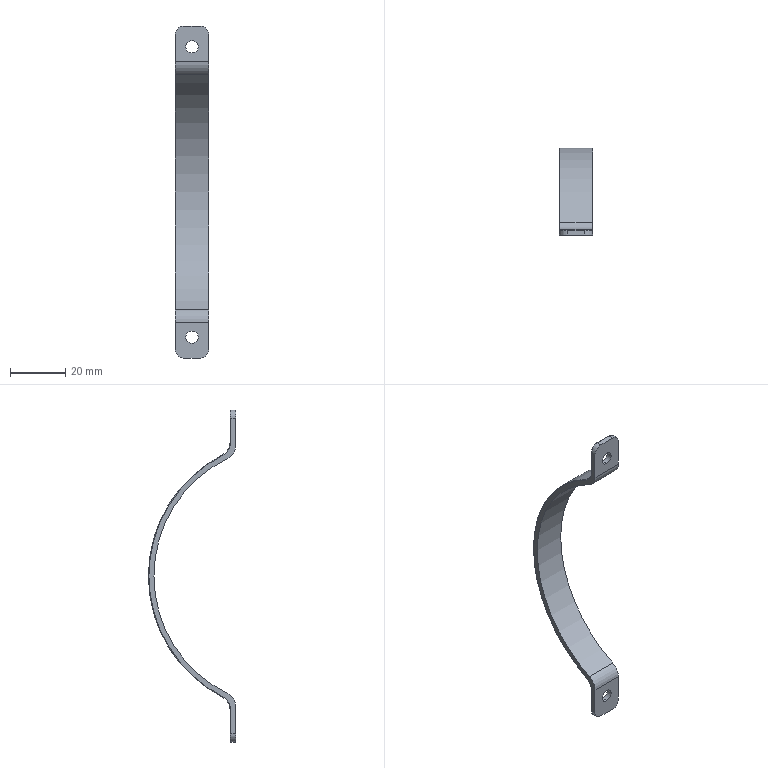Part | SolidWorks | features Fillet 4, Extrusion 1, ICE 1 | 1 solid | 38 faces | box 12 x 31.537 x 120 mm | volume 3389 mm3 | cylinder 20 | torus 10 | plane 8 | commonest cylinder face diameters 0.4 x6 4.5 x4 6 x4 10 x4 94.373 x1 98.392 x1
STEP:
#1=CARTESIAN_POINT('',(0.,17.659,-54.75));
#2=VERTEX_POINT('',#1);
#3=CARTESIAN_POINT('',(0.,17.659,-50.25));
#4=VERTEX_POINT('',#3);
#5=CARTESIAN_POINT('',(0.,17.659,-52.5));
#6=DIRECTION('',(0.,1.,0.));
#7=DIRECTION('',(0.,0.,1.));
#8=AXIS2_PLACEMENT_3D('',#5,#6,#7);
#9=CIRCLE('',#8,2.25);
#10=EDGE_CURVE('',#2,#4,#9,.T.);
#11=ORIENTED_EDGE('',*,*,#10,.F.);
#12=CARTESIAN_POINT('',(0.,19.659,-54.75));
#13=VERTEX_POINT('',#12);
#14=CARTESIAN_POINT('',(0.,7.659,-54.75));
#15=DIRECTION('',(0.,1.,0.));
#16=VECTOR('',#15,1000.);
#17=LINE('',#14,#16);
#18=EDGE_CURVE('',#2,#13,#17,.T.);
#19=ORIENTED_EDGE('',*,*,#18,.T.);
#20=CARTESIAN_POINT('',(0.,19.659,-50.25));
#21=VERTEX_POINT('',#20);
#22=CARTESIAN_POINT('',(0.,19.659,-52.5));
#23=DIRECTION('',(0.,1.,0.));
#24=DIRECTION('',(0.,0.,-1.));
#25=AXIS2_PLACEMENT_3D('',#22,#23,#24);
#26=CIRCLE('',#25,2.25);
#27=EDGE_CURVE('',#13,#21,#26,.T.);
#28=ORIENTED_EDGE('',*,*,#27,.T.);
#29=CARTESIAN_POINT('',(0.,7.659,-50.25));
#30=DIRECTION('',(0.,1.,0.));
#31=VECTOR('',#30,1000.);
#32=LINE('',#29,#31);
#33=EDGE_CURVE('',#4,#21,#32,.T.);
#34=ORIENTED_EDGE('',*,*,#33,.F.);
#35=EDGE_LOOP('',(#11,#19,#28,#34));
#36=FACE_OUTER_BOUND('',#35,.T.);
#37=CARTESIAN_POINT('',(0.,7.659,-52.5));
#38=DIRECTION('',(0.,1.,0.));
#39=DIRECTION('',(0.,0.,1.));
#40=AXIS2_PLACEMENT_3D('',#37,#38,#39);
#41=CYLINDRICAL_SURFACE('',#40,2.25);
#42=ADVANCED_FACE('',(#36),#41,.F.);
#43=CARTESIAN_POINT('',(0.,17.659,50.25));
#44=VERTEX_POINT('',#43);
#45=CARTESIAN_POINT('',(0.,17.659,54.75));
#46=VERTEX_POINT('',#45);
#47=CARTESIAN_POINT('',(0.,17.659,52.5));
#48=DIRECTION('',(0.,1.,0.));
#49=DIRECTION('',(0.,0.,1.));
#50=AXIS2_PLACEMENT_3D('',#47,#48,#49);
#51=CIRCLE('',#50,2.25);
#52=EDGE_CURVE('',#44,#46,#51,.T.);
#53=ORIENTED_EDGE('',*,*,#52,.F.);
#54=CARTESIAN_POINT('',(0.,19.659,50.25));
#55=VERTEX_POINT('',#54);
#56=CARTESIAN_POINT('',(0.,7.659,50.25));
#57=DIRECTION('',(0.,1.,0.));
#58=VECTOR('',#57,1000.);
#59=LINE('',#56,#58);
#60=EDGE_CURVE('',#44,#55,#59,.T.);
#61=ORIENTED_EDGE('',*,*,#60,.T.);
#62=CARTESIAN_POINT('',(0.,19.659,54.75));
#63=VERTEX_POINT('',#62);
#64=CARTESIAN_POINT('',(0.,19.659,52.5));
#65=DIRECTION('',(0.,1.,0.));
#66=DIRECTION('',(0.,0.,1.));
#67=AXIS2_PLACEMENT_3D('',#64,#65,#66);
#68=CIRCLE('',#67,2.25);
#69=EDGE_CURVE('',#55,#63,#68,.T.);
#70=ORIENTED_EDGE('',*,*,#69,.T.);
#71=CARTESIAN_POINT('',(0.,7.659,54.75));
#72=DIRECTION('',(0.,1.,0.));
#73=VECTOR('',#72,1000.);
#74=LINE('',#71,#73);
#75=EDGE_CURVE('',#46,#63,#74,.T.);
#76=ORIENTED_EDGE('',*,*,#75,.F.);
#77=EDGE_LOOP('',(#53,#61,#70,#76));
#78=FACE_OUTER_BOUND('',#77,.T.);
#79=CARTESIAN_POINT('',(0.,7.659,52.5));
#80=DIRECTION('',(0.,1.,0.));
#81=DIRECTION('',(0.,0.,1.));
#82=AXIS2_PLACEMENT_3D('',#79,#80,#81);
#83=CYLINDRICAL_SURFACE('',#82,2.25);
#84=ADVANCED_FACE('',(#78),#83,.F.);
#85=CARTESIAN_POINT('',(6.,20.488,42.506));
#86=VERTEX_POINT('',#85);
#87=CARTESIAN_POINT('',(6.,20.488,-42.506));
#88=VERTEX_POINT('',#87);
#89=CARTESIAN_POINT('',(6.,0.,0.));
#90=DIRECTION('',(-1.,0.,0.));
#91=DIRECTION('',(0.,0.,-1.));
#92=AXIS2_PLACEMENT_3D('',#89,#90,#91);
#93=CIRCLE('',#92,47.186);
#94=EDGE_CURVE('',#86,#88,#93,.T.);
#95=ORIENTED_EDGE('',*,*,#94,.F.);
#96=CARTESIAN_POINT('',(-6.,20.488,42.506));
#97=VERTEX_POINT('',#96);
#98=CARTESIAN_POINT('',(6.,20.488,42.506));
#99=DIRECTION('',(-1.,0.,0.));
#100=VECTOR('',#99,1000.);
#101=LINE('',#98,#100);
#102=EDGE_CURVE('',#86,#97,#101,.T.);
#103=ORIENTED_EDGE('',*,*,#102,.T.);
#104=CARTESIAN_POINT('',(-6.,20.488,-42.506));
#105=VERTEX_POINT('',#104);
#106=CARTESIAN_POINT('',(-6.,0.,0.));
#107=DIRECTION('',(-1.,0.,0.));
#108=DIRECTION('',(0.,0.,-1.));
#109=AXIS2_PLACEMENT_3D('',#106,#107,#108);
#110=CIRCLE('',#109,47.186);
#111=EDGE_CURVE('',#97,#105,#110,.T.);
#112=ORIENTED_EDGE('',*,*,#111,.T.);
#113=CARTESIAN_POINT('',(6.,20.488,-42.506));
#114=DIRECTION('',(1.,0.,0.));
#115=VECTOR('',#114,1000.);
#116=LINE('',#113,#115);
#117=EDGE_CURVE('',#105,#88,#116,.T.);
#118=ORIENTED_EDGE('',*,*,#117,.T.);
#119=EDGE_LOOP('',(#95,#103,#112,#118));
#120=FACE_OUTER_BOUND('',#119,.T.);
#121=CARTESIAN_POINT('',(6.,0.,0.));
#122=DIRECTION('',(-1.,0.,0.));
#123=DIRECTION('',(0.,0.,1.));
#124=AXIS2_PLACEMENT_3D('',#121,#122,#123);
#125=CYLINDRICAL_SURFACE('',#124,47.186);
#126=ADVANCED_FACE('',(#120),#125,.F.);
#127=CARTESIAN_POINT('',(0.,17.659,-52.5));
#128=DIRECTION('',(0.,1.,0.));
#129=DIRECTION('',(0.,0.,1.));
#130=AXIS2_PLACEMENT_3D('',#127,#128,#129);
#131=CIRCLE('',#130,2.25);
#132=EDGE_CURVE('',#4,#2,#131,.T.);
#133=ORIENTED_EDGE('',*,*,#132,.T.);
#134=ORIENTED_EDGE('',*,*,#10,.T.);
#135=EDGE_LOOP('',(#133,#134));
#136=FACE_BOUND('',#135,.T.);
#137=CARTESIAN_POINT('',(6.,17.659,-47.01));
#138=VERTEX_POINT('',#137);
#139=CARTESIAN_POINT('',(6.,17.659,-57.));
#140=VERTEX_POINT('',#139);
#141=CARTESIAN_POINT('',(6.,17.659,-43.757));
#142=DIRECTION('',(0.,0.,-1.));
#143=VECTOR('',#142,1000.);
#144=LINE('',#141,#143);
#145=EDGE_CURVE('',#138,#140,#144,.T.);
#146=ORIENTED_EDGE('',*,*,#145,.F.);
#147=CARTESIAN_POINT('',(-6.,17.659,-47.01));
#148=VERTEX_POINT('',#147);
#149=CARTESIAN_POINT('',(6.,17.659,-47.01));
#150=DIRECTION('',(-1.,0.,0.));
#151=VECTOR('',#150,1000.);
#152=LINE('',#149,#151);
#153=EDGE_CURVE('',#138,#148,#152,.T.);
#154=ORIENTED_EDGE('',*,*,#153,.T.);
#155=CARTESIAN_POINT('',(-6.,17.659,-57.));
#156=VERTEX_POINT('',#155);
#157=CARTESIAN_POINT('',(-6.,17.659,-43.757));
#158=DIRECTION('',(0.,0.,-1.));
#159=VECTOR('',#158,1000.);
#160=LINE('',#157,#159);
#161=EDGE_CURVE('',#148,#156,#160,.T.);
#162=ORIENTED_EDGE('',*,*,#161,.T.);
#163=CARTESIAN_POINT('',(-3.,17.659,-60.));
#164=VERTEX_POINT('',#163);
#165=CARTESIAN_POINT('',(-3.,17.659,-57.));
#166=DIRECTION('',(0.,-1.,0.));
#167=DIRECTION('',(0.,0.,1.));
#168=AXIS2_PLACEMENT_3D('',#165,#166,#167);
#169=CIRCLE('',#168,3.);
#170=EDGE_CURVE('',#156,#164,#169,.T.);
#171=ORIENTED_EDGE('',*,*,#170,.T.);
#172=CARTESIAN_POINT('',(3.,17.659,-60.));
#173=VERTEX_POINT('',#172);
#174=CARTESIAN_POINT('',(6.,17.659,-60.));
#175=DIRECTION('',(-1.,0.,0.));
#176=VECTOR('',#175,1000.);
#177=LINE('',#174,#176);
#178=EDGE_CURVE('',#173,#164,#177,.T.);
#179=ORIENTED_EDGE('',*,*,#178,.F.);
#180=CARTESIAN_POINT('',(3.,17.659,-57.));
#181=DIRECTION('',(0.,-1.,0.));
#182=DIRECTION('',(0.,0.,1.));
#183=AXIS2_PLACEMENT_3D('',#180,#181,#182);
#184=CIRCLE('',#183,3.);
#185=EDGE_CURVE('',#173,#140,#184,.T.);
#186=ORIENTED_EDGE('',*,*,#185,.T.);
#187=EDGE_LOOP('',(#146,#154,#162,#171,#179,#186));
#188=FACE_OUTER_BOUND('',#187,.T.);
#189=CARTESIAN_POINT('',(6.,17.659,-43.757));
#190=DIRECTION('',(0.,1.,0.));
#191=DIRECTION('',(0.,0.,1.));
#192=AXIS2_PLACEMENT_3D('',#189,#190,#191);
#193=PLANE('',#192);
#194=ADVANCED_FACE('',(#136,#188),#193,.F.);
#195=CARTESIAN_POINT('',(-3.,19.459,-60.));
#196=VERTEX_POINT('',#195);
#197=CARTESIAN_POINT('',(-3.,19.659,-60.));
#198=DIRECTION('',(0.,1.,0.));
#199=VECTOR('',#198,1000.);
#200=LINE('',#197,#199);
#201=EDGE_CURVE('',#164,#196,#200,.T.);
#202=ORIENTED_EDGE('',*,*,#201,.T.);
#203=CARTESIAN_POINT('',(3.,19.459,-60.));
#204=VERTEX_POINT('',#203);
#205=CARTESIAN_POINT('',(6.,19.459,-60.));
#206=DIRECTION('',(1.,0.,0.));
#207=VECTOR('',#206,1000.);
#208=LINE('',#205,#207);
#209=EDGE_CURVE('',#196,#204,#208,.T.);
#210=ORIENTED_EDGE('',*,*,#209,.T.);
#211=CARTESIAN_POINT('',(3.,17.659,-60.));
#212=DIRECTION('',(0.,-1.,0.));
#213=VECTOR('',#212,1000.);
#214=LINE('',#211,#213);
#215=EDGE_CURVE('',#204,#173,#214,.T.);
#216=ORIENTED_EDGE('',*,*,#215,.T.);
#217=ORIENTED_EDGE('',*,*,#178,.T.);
#218=EDGE_LOOP('',(#202,#210,#216,#217));
#219=FACE_OUTER_BOUND('',#218,.T.);
#220=CARTESIAN_POINT('',(6.,19.659,-60.));
#221=DIRECTION('',(0.,0.,1.));
#222=DIRECTION('',(0.,-1.,0.));
#223=AXIS2_PLACEMENT_3D('',#220,#221,#222);
#224=PLANE('',#223);
#225=ADVANCED_FACE('',(#219),#224,.F.);
#226=CARTESIAN_POINT('',(0.,19.659,-52.5));
#227=DIRECTION('',(0.,1.,0.));
#228=DIRECTION('',(0.,0.,-1.));
#229=AXIS2_PLACEMENT_3D('',#226,#227,#228);
#230=CIRCLE('',#229,2.25);
#231=EDGE_CURVE('',#21,#13,#230,.T.);
#232=ORIENTED_EDGE('',*,*,#231,.F.);
#233=ORIENTED_EDGE('',*,*,#27,.F.);
#234=EDGE_LOOP('',(#232,#233));
#235=FACE_BOUND('',#234,.T.);
#236=CARTESIAN_POINT('',(-5.8,19.659,-48.261));
#237=VERTEX_POINT('',#236);
#238=CARTESIAN_POINT('',(5.8,19.659,-48.261));
#239=VERTEX_POINT('',#238);
#240=CARTESIAN_POINT('',(6.,19.659,-48.261));
#241=DIRECTION('',(1.,0.,0.));
#242=VECTOR('',#241,1000.);
#243=LINE('',#240,#242);
#244=EDGE_CURVE('',#237,#239,#243,.T.);
#245=ORIENTED_EDGE('',*,*,#244,.T.);
#246=CARTESIAN_POINT('',(5.8,19.659,-57.));
#247=VERTEX_POINT('',#246);
#248=CARTESIAN_POINT('',(5.8,19.659,-57.));
#249=DIRECTION('',(0.,0.,-1.));
#250=VECTOR('',#249,1000.);
#251=LINE('',#248,#250);
#252=EDGE_CURVE('',#239,#247,#251,.T.);
#253=ORIENTED_EDGE('',*,*,#252,.T.);
#254=CARTESIAN_POINT('',(3.,19.659,-59.8));
#255=VERTEX_POINT('',#254);
#256=CARTESIAN_POINT('',(3.,19.659,-57.));
#257=DIRECTION('',(0.,1.,0.));
#258=DIRECTION('',(0.,0.,-1.));
#259=AXIS2_PLACEMENT_3D('',#256,#257,#258);
#260=CIRCLE('',#259,2.8);
#261=EDGE_CURVE('',#247,#255,#260,.T.);
#262=ORIENTED_EDGE('',*,*,#261,.T.);
#263=CARTESIAN_POINT('',(-3.,19.659,-59.8));
#264=VERTEX_POINT('',#263);
#265=CARTESIAN_POINT('',(6.,19.659,-59.8));
#266=DIRECTION('',(-1.,0.,0.));
#267=VECTOR('',#266,1000.);
#268=LINE('',#265,#267);
#269=EDGE_CURVE('',#255,#264,#268,.T.);
#270=ORIENTED_EDGE('',*,*,#269,.T.);
#271=CARTESIAN_POINT('',(-5.8,19.659,-57.));
#272=VERTEX_POINT('',#271);
#273=CARTESIAN_POINT('',(-3.,19.659,-57.));
#274=DIRECTION('',(0.,1.,0.));
#275=DIRECTION('',(0.,0.,-1.));
#276=AXIS2_PLACEMENT_3D('',#273,#274,#275);
#277=CIRCLE('',#276,2.8);
#278=EDGE_CURVE('',#264,#272,#277,.T.);
#279=ORIENTED_EDGE('',*,*,#278,.T.);
#280=CARTESIAN_POINT('',(-5.8,19.659,-45.097));
#281=DIRECTION('',(0.,0.,1.));
#282=VECTOR('',#281,1000.);
#283=LINE('',#280,#282);
#284=EDGE_CURVE('',#272,#237,#283,.T.);
#285=ORIENTED_EDGE('',*,*,#284,.T.);
#286=EDGE_LOOP('',(#245,#253,#262,#270,#279,#285));
#287=FACE_OUTER_BOUND('',#286,.T.);
#288=CARTESIAN_POINT('',(6.,19.659,-45.097));
#289=DIRECTION('',(0.,-1.,0.));
#290=DIRECTION('',(0.,0.,-1.));
#291=AXIS2_PLACEMENT_3D('',#288,#289,#290);
#292=PLANE('',#291);
#293=ADVANCED_FACE('',(#235,#287),#292,.F.);
#294=CARTESIAN_POINT('',(5.8,22.384,-43.808));
#295=VERTEX_POINT('',#294);
#296=CARTESIAN_POINT('',(-5.8,22.384,-43.808));
#297=VERTEX_POINT('',#296);
#298=CARTESIAN_POINT('',(6.,22.384,-43.808));
#299=DIRECTION('',(-1.,0.,0.));
#300=VECTOR('',#299,1000.);
#301=LINE('',#298,#300);
#302=EDGE_CURVE('',#295,#297,#301,.T.);
#303=ORIENTED_EDGE('',*,*,#302,.T.);
#304=CARTESIAN_POINT('',(-5.8,22.384,43.808));
#305=VERTEX_POINT('',#304);
#306=CARTESIAN_POINT('',(-5.8,0.,0.));
#307=DIRECTION('',(1.,0.,0.));
#308=DIRECTION('',(0.,0.,-1.));
#309=AXIS2_PLACEMENT_3D('',#306,#307,#308);
#310=CIRCLE('',#309,49.196);
#311=EDGE_CURVE('',#297,#305,#310,.T.);
#312=ORIENTED_EDGE('',*,*,#311,.T.);
#313=CARTESIAN_POINT('',(5.8,22.384,43.808));
#314=VERTEX_POINT('',#313);
#315=CARTESIAN_POINT('',(6.,22.384,43.808));
#316=DIRECTION('',(1.,0.,0.));
#317=VECTOR('',#316,1000.);
#318=LINE('',#315,#317);
#319=EDGE_CURVE('',#305,#314,#318,.T.);
#320=ORIENTED_EDGE('',*,*,#319,.T.);
#321=CARTESIAN_POINT('',(5.8,0.,0.));
#322=DIRECTION('',(-1.,0.,0.));
#323=DIRECTION('',(0.,0.,-1.));
#324=AXIS2_PLACEMENT_3D('',#321,#322,#323);
#325=CIRCLE('',#324,49.196);
#326=EDGE_CURVE('',#314,#295,#325,.T.);
#327=ORIENTED_EDGE('',*,*,#326,.T.);
#328=EDGE_LOOP('',(#303,#312,#320,#327));
#329=FACE_OUTER_BOUND('',#328,.T.);
#330=CARTESIAN_POINT('',(6.,0.,0.));
#331=DIRECTION('',(-1.,0.,0.));
#332=DIRECTION('',(0.,0.,1.));
#333=AXIS2_PLACEMENT_3D('',#330,#331,#332);
#334=CYLINDRICAL_SURFACE('',#333,49.196);
#335=ADVANCED_FACE('',(#329),#334,.T.);
#336=CARTESIAN_POINT('',(0.,19.659,52.5));
#337=DIRECTION('',(0.,1.,0.));
#338=DIRECTION('',(0.,0.,1.));
#339=AXIS2_PLACEMENT_3D('',#336,#337,#338);
#340=CIRCLE('',#339,2.25);
#341=EDGE_CURVE('',#63,#55,#340,.T.);
#342=ORIENTED_EDGE('',*,*,#341,.F.);
#343=ORIENTED_EDGE('',*,*,#69,.F.);
#344=EDGE_LOOP('',(#342,#343));
#345=FACE_BOUND('',#344,.T.);
#346=CARTESIAN_POINT('',(5.8,19.659,48.261));
#347=VERTEX_POINT('',#346);
#348=CARTESIAN_POINT('',(-5.8,19.659,48.261));
#349=VERTEX_POINT('',#348);
#350=CARTESIAN_POINT('',(-6.,19.659,48.261));
#351=DIRECTION('',(-1.,0.,0.));
#352=VECTOR('',#351,1000.);
#353=LINE('',#350,#352);
#354=EDGE_CURVE('',#347,#349,#353,.T.);
#355=ORIENTED_EDGE('',*,*,#354,.T.);
#356=CARTESIAN_POINT('',(-5.8,19.659,57.));
#357=VERTEX_POINT('',#356);
#358=CARTESIAN_POINT('',(-5.8,19.659,45.097));
#359=DIRECTION('',(0.,0.,1.));
#360=VECTOR('',#359,1000.);
#361=LINE('',#358,#360);
#362=EDGE_CURVE('',#349,#357,#361,.T.);
#363=ORIENTED_EDGE('',*,*,#362,.T.);
#364=CARTESIAN_POINT('',(-3.,19.659,59.8));
#365=VERTEX_POINT('',#364);
#366=CARTESIAN_POINT('',(-3.,19.659,57.));
#367=DIRECTION('',(0.,1.,0.));
#368=DIRECTION('',(0.,0.,-1.));
#369=AXIS2_PLACEMENT_3D('',#366,#367,#368);
#370=CIRCLE('',#369,2.8);
#371=EDGE_CURVE('',#357,#365,#370,.T.);
#372=ORIENTED_EDGE('',*,*,#371,.T.);
#373=CARTESIAN_POINT('',(3.,19.659,59.8));
#374=VERTEX_POINT('',#373);
#375=CARTESIAN_POINT('',(6.,19.659,59.8));
#376=DIRECTION('',(1.,0.,0.));
#377=VECTOR('',#376,1000.);
#378=LINE('',#375,#377);
#379=EDGE_CURVE('',#365,#374,#378,.T.);
#380=ORIENTED_EDGE('',*,*,#379,.T.);
#381=CARTESIAN_POINT('',(5.8,19.659,57.));
#382=VERTEX_POINT('',#381);
#383=CARTESIAN_POINT('',(3.,19.659,57.));
#384=DIRECTION('',(0.,1.,0.));
#385=DIRECTION('',(0.,0.,-1.));
#386=AXIS2_PLACEMENT_3D('',#383,#384,#385);
#387=CIRCLE('',#386,2.8);
#388=EDGE_CURVE('',#374,#382,#387,.T.);
#389=ORIENTED_EDGE('',*,*,#388,.T.);
#390=CARTESIAN_POINT('',(5.8,19.659,48.261));
#391=DIRECTION('',(0.,0.,-1.));
#392=VECTOR('',#391,1000.);
#393=LINE('',#390,#392);
#394=EDGE_CURVE('',#382,#347,#393,.T.);
#395=ORIENTED_EDGE('',*,*,#394,.T.);
#396=EDGE_LOOP('',(#355,#363,#372,#380,#389,#395));
#397=FACE_OUTER_BOUND('',#396,.T.);
#398=CARTESIAN_POINT('',(6.,19.659,45.097));
#399=DIRECTION('',(0.,-1.,0.));
#400=DIRECTION('',(0.,0.,-1.));
#401=AXIS2_PLACEMENT_3D('',#398,#399,#400);
#402=PLANE('',#401);
#403=ADVANCED_FACE('',(#345,#397),#402,.F.);
#404=CARTESIAN_POINT('',(3.,17.659,60.));
#405=VERTEX_POINT('',#404);
#406=CARTESIAN_POINT('',(3.,19.459,60.));
#407=VERTEX_POINT('',#406);
#408=CARTESIAN_POINT('',(3.,19.659,60.));
#409=DIRECTION('',(0.,1.,0.));
#410=VECTOR('',#409,1000.);
#411=LINE('',#408,#410);
#412=EDGE_CURVE('',#405,#407,#411,.T.);
#413=ORIENTED_EDGE('',*,*,#412,.T.);
#414=CARTESIAN_POINT('',(-3.,19.459,60.));
#415=VERTEX_POINT('',#414);
#416=CARTESIAN_POINT('',(6.,19.459,60.));
#417=DIRECTION('',(-1.,0.,0.));
#418=VECTOR('',#417,1000.);
#419=LINE('',#416,#418);
#420=EDGE_CURVE('',#407,#415,#419,.T.);
#421=ORIENTED_EDGE('',*,*,#420,.T.);
#422=CARTESIAN_POINT('',(-3.,17.659,60.));
#423=VERTEX_POINT('',#422);
#424=CARTESIAN_POINT('',(-3.,19.659,60.));
#425=DIRECTION('',(0.,-1.,0.));
#426=VECTOR('',#425,1000.);
#427=LINE('',#424,#426);
#428=EDGE_CURVE('',#415,#423,#427,.T.);
#429=ORIENTED_EDGE('',*,*,#428,.T.);
#430=CARTESIAN_POINT('',(6.,17.659,60.));
#431=DIRECTION('',(-1.,0.,0.));
#432=VECTOR('',#431,1000.);
#433=LINE('',#430,#432);
#434=EDGE_CURVE('',#405,#423,#433,.T.);
#435=ORIENTED_EDGE('',*,*,#434,.F.);
#436=EDGE_LOOP('',(#413,#421,#429,#435));
#437=FACE_OUTER_BOUND('',#436,.T.);
#438=CARTESIAN_POINT('',(6.,19.659,60.));
#439=DIRECTION('',(0.,0.,-1.));
#440=DIRECTION('',(0.,1.,0.));
#441=AXIS2_PLACEMENT_3D('',#438,#439,#440);
#442=PLANE('',#441);
#443=ADVANCED_FACE('',(#437),#442,.F.);
#444=CARTESIAN_POINT('',(0.,17.659,52.5));
#445=DIRECTION('',(0.,1.,0.));
#446=DIRECTION('',(0.,0.,1.));
#447=AXIS2_PLACEMENT_3D('',#444,#445,#446);
#448=CIRCLE('',#447,2.25);
#449=EDGE_CURVE('',#46,#44,#448,.T.);
#450=ORIENTED_EDGE('',*,*,#449,.T.);
#451=ORIENTED_EDGE('',*,*,#52,.T.);
#452=EDGE_LOOP('',(#450,#451));
#453=FACE_BOUND('',#452,.T.);
#454=CARTESIAN_POINT('',(-6.,17.659,57.));
#455=VERTEX_POINT('',#454);
#456=CARTESIAN_POINT('',(-6.,17.659,47.01));
#457=VERTEX_POINT('',#456);
#458=CARTESIAN_POINT('',(-6.,17.659,43.757));
#459=DIRECTION('',(0.,0.,-1.));
#460=VECTOR('',#459,1000.);
#461=LINE('',#458,#460);
#462=EDGE_CURVE('',#455,#457,#461,.T.);
#463=ORIENTED_EDGE('',*,*,#462,.T.);
#464=CARTESIAN_POINT('',(6.,17.659,47.01));
#465=VERTEX_POINT('',#464);
#466=CARTESIAN_POINT('',(6.,17.659,47.01));
#467=DIRECTION('',(1.,0.,0.));
#468=VECTOR('',#467,1000.);
#469=LINE('',#466,#468);
#470=EDGE_CURVE('',#457,#465,#469,.T.);
#471=ORIENTED_EDGE('',*,*,#470,.T.);
#472=CARTESIAN_POINT('',(6.,17.659,57.));
#473=VERTEX_POINT('',#472);
#474=CARTESIAN_POINT('',(6.,17.659,43.757));
#475=DIRECTION('',(0.,0.,-1.));
#476=VECTOR('',#475,1000.);
#477=LINE('',#474,#476);
#478=EDGE_CURVE('',#473,#465,#477,.T.);
#479=ORIENTED_EDGE('',*,*,#478,.F.);
#480=CARTESIAN_POINT('',(3.,17.659,57.));
#481=DIRECTION('',(0.,-1.,0.));
#482=DIRECTION('',(0.,0.,1.));
#483=AXIS2_PLACEMENT_3D('',#480,#481,#482);
#484=CIRCLE('',#483,3.);
#485=EDGE_CURVE('',#473,#405,#484,.T.);
#486=ORIENTED_EDGE('',*,*,#485,.T.);
#487=ORIENTED_EDGE('',*,*,#434,.T.);
#488=CARTESIAN_POINT('',(-3.,17.659,57.));
#489=DIRECTION('',(0.,-1.,0.));
#490=DIRECTION('',(0.,0.,1.));
#491=AXIS2_PLACEMENT_3D('',#488,#489,#490);
#492=CIRCLE('',#491,3.);
#493=EDGE_CURVE('',#423,#455,#492,.T.);
#494=ORIENTED_EDGE('',*,*,#493,.T.);
#495=EDGE_LOOP('',(#463,#471,#479,#486,#487,#494));
#496=FACE_OUTER_BOUND('',#495,.T.);
#497=CARTESIAN_POINT('',(6.,17.659,43.757));
#498=DIRECTION('',(0.,1.,0.));
#499=DIRECTION('',(0.,0.,1.));
#500=AXIS2_PLACEMENT_3D('',#497,#498,#499);
#501=PLANE('',#500);
#502=ADVANCED_FACE('',(#453,#496),#501,.F.);
#503=CARTESIAN_POINT('',(6.,19.459,-57.));
#504=VERTEX_POINT('',#503);
#505=CARTESIAN_POINT('',(6.,19.659,-57.));
#506=DIRECTION('',(0.,1.,0.));
#507=VECTOR('',#506,1000.);
#508=LINE('',#505,#507);
#509=EDGE_CURVE('',#140,#504,#508,.T.);
#510=ORIENTED_EDGE('',*,*,#509,.T.);
#511=CARTESIAN_POINT('',(6.,19.459,-48.261));
#512=VERTEX_POINT('',#511);
#513=CARTESIAN_POINT('',(6.,19.459,-48.261));
#514=DIRECTION('',(0.,0.,1.));
#515=VECTOR('',#514,1000.);
#516=LINE('',#513,#515);
#517=EDGE_CURVE('',#504,#512,#516,.T.);
#518=ORIENTED_EDGE('',*,*,#517,.T.);
#519=CARTESIAN_POINT('',(6.,22.293,-43.63));
#520=VERTEX_POINT('',#519);
#521=CARTESIAN_POINT('',(6.,24.659,-48.261));
#522=DIRECTION('',(-1.,0.,0.));
#523=DIRECTION('',(0.,0.,-1.));
#524=AXIS2_PLACEMENT_3D('',#521,#522,#523);
#525=CIRCLE('',#524,5.2);
#526=EDGE_CURVE('',#512,#520,#525,.T.);
#527=ORIENTED_EDGE('',*,*,#526,.T.);
#528=CARTESIAN_POINT('',(6.,22.293,43.63));
#529=VERTEX_POINT('',#528);
#530=CARTESIAN_POINT('',(6.,0.,0.));
#531=DIRECTION('',(1.,0.,0.));
#532=DIRECTION('',(0.,0.,-1.));
#533=AXIS2_PLACEMENT_3D('',#530,#531,#532);
#534=CIRCLE('',#533,48.996);
#535=EDGE_CURVE('',#520,#529,#534,.T.);
#536=ORIENTED_EDGE('',*,*,#535,.T.);
#537=CARTESIAN_POINT('',(6.,19.459,48.261));
#538=VERTEX_POINT('',#537);
#539=CARTESIAN_POINT('',(6.,24.659,48.261));
#540=DIRECTION('',(-1.,0.,0.));
#541=DIRECTION('',(0.,0.,-1.));
#542=AXIS2_PLACEMENT_3D('',#539,#540,#541);
#543=CIRCLE('',#542,5.2);
#544=EDGE_CURVE('',#529,#538,#543,.T.);
#545=ORIENTED_EDGE('',*,*,#544,.T.);
#546=CARTESIAN_POINT('',(6.,19.459,57.));
#547=VERTEX_POINT('',#546);
#548=CARTESIAN_POINT('',(6.,19.459,57.));
#549=DIRECTION('',(0.,0.,1.));
#550=VECTOR('',#549,1000.);
#551=LINE('',#548,#550);
#552=EDGE_CURVE('',#538,#547,#551,.T.);
#553=ORIENTED_EDGE('',*,*,#552,.T.);
#554=CARTESIAN_POINT('',(6.,17.659,57.));
#555=DIRECTION('',(0.,-1.,0.));
#556=VECTOR('',#555,1000.);
#557=LINE('',#554,#556);
#558=EDGE_CURVE('',#547,#473,#557,.T.);
#559=ORIENTED_EDGE('',*,*,#558,.T.);
#560=ORIENTED_EDGE('',*,*,#478,.T.);
#561=CARTESIAN_POINT('',(6.,22.659,47.01));
#562=DIRECTION('',(1.,0.,0.));
#563=DIRECTION('',(0.,0.,-1.));
#564=AXIS2_PLACEMENT_3D('',#561,#562,#563);
#565=CIRCLE('',#564,5.);
#566=EDGE_CURVE('',#465,#86,#565,.T.);
#567=ORIENTED_EDGE('',*,*,#566,.T.);
#568=ORIENTED_EDGE('',*,*,#94,.T.);
#569=CARTESIAN_POINT('',(6.,22.659,-47.01));
#570=DIRECTION('',(1.,0.,0.));
#571=DIRECTION('',(0.,0.,-1.));
#572=AXIS2_PLACEMENT_3D('',#569,#570,#571);
#573=CIRCLE('',#572,5.);
#574=EDGE_CURVE('',#88,#138,#573,.T.);
#575=ORIENTED_EDGE('',*,*,#574,.T.);
#576=ORIENTED_EDGE('',*,*,#145,.T.);
#577=EDGE_LOOP('',(#510,#518,#527,#536,#545,#553,#559,#560,#567,#568,#575,#576));
#578=FACE_OUTER_BOUND('',#577,.T.);
#579=CARTESIAN_POINT('',(6.,0.,0.));
#580=DIRECTION('',(1.,0.,0.));
#581=DIRECTION('',(0.,0.,-1.));
#582=AXIS2_PLACEMENT_3D('',#579,#580,#581);
#583=PLANE('',#582);
#584=ADVANCED_FACE('',(#578),#583,.T.);
#585=CARTESIAN_POINT('',(-6.,22.293,-43.63));
#586=VERTEX_POINT('',#585);
#587=CARTESIAN_POINT('',(-6.,19.459,-48.261));
#588=VERTEX_POINT('',#587);
#589=CARTESIAN_POINT('',(-6.,24.659,-48.261));
#590=DIRECTION('',(1.,0.,0.));
#591=DIRECTION('',(0.,0.,-1.));
#592=AXIS2_PLACEMENT_3D('',#589,#590,#591);
#593=CIRCLE('',#592,5.2);
#594=EDGE_CURVE('',#586,#588,#593,.T.);
#595=ORIENTED_EDGE('',*,*,#594,.T.);
#596=CARTESIAN_POINT('',(-6.,19.459,-57.));
#597=VERTEX_POINT('',#596);
#598=CARTESIAN_POINT('',(-6.,19.459,0.));
#599=DIRECTION('',(0.,0.,-1.));
#600=VECTOR('',#599,1000.);
#601=LINE('',#598,#600);
#602=EDGE_CURVE('',#588,#597,#601,.T.);
#603=ORIENTED_EDGE('',*,*,#602,.T.);
#604=CARTESIAN_POINT('',(-6.,0.,-57.));
#605=DIRECTION('',(0.,-1.,0.));
#606=VECTOR('',#605,1000.);
#607=LINE('',#604,#606);
#608=EDGE_CURVE('',#597,#156,#607,.T.);
#609=ORIENTED_EDGE('',*,*,#608,.T.);
#610=ORIENTED_EDGE('',*,*,#161,.F.);
#611=CARTESIAN_POINT('',(-6.,22.659,-47.01));
#612=DIRECTION('',(-1.,0.,0.));
#613=DIRECTION('',(0.,0.,-1.));
#614=AXIS2_PLACEMENT_3D('',#611,#612,#613);
#615=CIRCLE('',#614,5.);
#616=EDGE_CURVE('',#148,#105,#615,.T.);
#617=ORIENTED_EDGE('',*,*,#616,.T.);
#618=ORIENTED_EDGE('',*,*,#111,.F.);
#619=CARTESIAN_POINT('',(-6.,22.659,47.01));
#620=DIRECTION('',(-1.,0.,0.));
#621=DIRECTION('',(0.,0.,-1.));
#622=AXIS2_PLACEMENT_3D('',#619,#620,#621);
#623=CIRCLE('',#622,5.);
#624=EDGE_CURVE('',#97,#457,#623,.T.);
#625=ORIENTED_EDGE('',*,*,#624,.T.);
#626=ORIENTED_EDGE('',*,*,#462,.F.);
#627=CARTESIAN_POINT('',(-6.,19.459,57.));
#628=VERTEX_POINT('',#627);
#629=CARTESIAN_POINT('',(-6.,0.,57.));
#630=DIRECTION('',(0.,1.,0.));
#631=VECTOR('',#630,1000.);
#632=LINE('',#629,#631);
#633=EDGE_CURVE('',#455,#628,#632,.T.);
#634=ORIENTED_EDGE('',*,*,#633,.T.);
#635=CARTESIAN_POINT('',(-6.,19.459,48.261));
#636=VERTEX_POINT('',#635);
#637=CARTESIAN_POINT('',(-6.,19.459,0.));
#638=DIRECTION('',(0.,0.,-1.));
#639=VECTOR('',#638,1000.);
#640=LINE('',#637,#639);
#641=EDGE_CURVE('',#628,#636,#640,.T.);
#642=ORIENTED_EDGE('',*,*,#641,.T.);
#643=CARTESIAN_POINT('',(-6.,22.293,43.63));
#644=VERTEX_POINT('',#643);
#645=CARTESIAN_POINT('',(-6.,24.659,48.261));
#646=DIRECTION('',(1.,0.,0.));
#647=DIRECTION('',(0.,0.,-1.));
#648=AXIS2_PLACEMENT_3D('',#645,#646,#647);
#649=CIRCLE('',#648,5.2);
#650=EDGE_CURVE('',#636,#644,#649,.T.);
#651=ORIENTED_EDGE('',*,*,#650,.T.);
#652=CARTESIAN_POINT('',(-6.,0.,0.));
#653=DIRECTION('',(-1.,0.,0.));
#654=DIRECTION('',(0.,0.,-1.));
#655=AXIS2_PLACEMENT_3D('',#652,#653,#654);
#656=CIRCLE('',#655,48.996);
#657=EDGE_CURVE('',#644,#586,#656,.T.);
#658=ORIENTED_EDGE('',*,*,#657,.T.);
#659=EDGE_LOOP('',(#595,#603,#609,#610,#617,#618,#625,#626,#634,#642,#651,#658));
#660=FACE_OUTER_BOUND('',#659,.T.);
#661=CARTESIAN_POINT('',(-6.,0.,0.));
#662=DIRECTION('',(1.,0.,0.));
#663=DIRECTION('',(0.,0.,-1.));
#664=AXIS2_PLACEMENT_3D('',#661,#662,#663);
#665=PLANE('',#664);
#666=ADVANCED_FACE('',(#660),#665,.F.);
#667=ORIENTED_EDGE('',*,*,#60,.F.);
#668=ORIENTED_EDGE('',*,*,#449,.F.);
#669=ORIENTED_EDGE('',*,*,#75,.T.);
#670=ORIENTED_EDGE('',*,*,#341,.T.);
#671=EDGE_LOOP('',(#667,#668,#669,#670));
#672=FACE_OUTER_BOUND('',#671,.T.);
#673=CARTESIAN_POINT('',(0.,7.659,52.5));
#674=DIRECTION('',(0.,1.,0.));
#675=DIRECTION('',(0.,0.,1.));
#676=AXIS2_PLACEMENT_3D('',#673,#674,#675);
#677=CYLINDRICAL_SURFACE('',#676,2.25);
#678=ADVANCED_FACE('',(#672),#677,.F.);
#679=ORIENTED_EDGE('',*,*,#18,.F.);
#680=ORIENTED_EDGE('',*,*,#132,.F.);
#681=ORIENTED_EDGE('',*,*,#33,.T.);
#682=ORIENTED_EDGE('',*,*,#231,.T.);
#683=EDGE_LOOP('',(#679,#680,#681,#682));
#684=FACE_OUTER_BOUND('',#683,.T.);
#685=CARTESIAN_POINT('',(0.,7.659,-52.5));
#686=DIRECTION('',(0.,1.,0.));
#687=DIRECTION('',(0.,0.,1.));
#688=AXIS2_PLACEMENT_3D('',#685,#686,#687);
#689=CYLINDRICAL_SURFACE('',#688,2.25);
#690=ADVANCED_FACE('',(#684),#689,.F.);
#691=ORIENTED_EDGE('',*,*,#558,.F.);
#692=CARTESIAN_POINT('',(3.,19.459,57.));
#693=DIRECTION('',(0.,-1.,0.));
#694=DIRECTION('',(0.,0.,-1.));
#695=AXIS2_PLACEMENT_3D('',#692,#693,#694);
#696=CIRCLE('',#695,3.);
#697=EDGE_CURVE('',#547,#407,#696,.T.);
#698=ORIENTED_EDGE('',*,*,#697,.T.);
#699=ORIENTED_EDGE('',*,*,#412,.F.);
#700=ORIENTED_EDGE('',*,*,#485,.F.);
#701=EDGE_LOOP('',(#691,#698,#699,#700));
#702=FACE_OUTER_BOUND('',#701,.T.);
#703=CARTESIAN_POINT('',(3.,0.,57.));
#704=DIRECTION('',(0.,1.,0.));
#705=DIRECTION('',(0.,0.,1.));
#706=AXIS2_PLACEMENT_3D('',#703,#704,#705);
#707=CYLINDRICAL_SURFACE('',#706,3.);
#708=ADVANCED_FACE('',(#702),#707,.T.);
#709=ORIENTED_EDGE('',*,*,#428,.F.);
#710=CARTESIAN_POINT('',(-3.,19.459,57.));
#711=DIRECTION('',(0.,-1.,0.));
#712=DIRECTION('',(0.,0.,-1.));
#713=AXIS2_PLACEMENT_3D('',#710,#711,#712);
#714=CIRCLE('',#713,3.);
#715=EDGE_CURVE('',#415,#628,#714,.T.);
#716=ORIENTED_EDGE('',*,*,#715,.T.);
#717=ORIENTED_EDGE('',*,*,#633,.F.);
#718=ORIENTED_EDGE('',*,*,#493,.F.);
#719=EDGE_LOOP('',(#709,#716,#717,#718));
#720=FACE_OUTER_BOUND('',#719,.T.);
#721=CARTESIAN_POINT('',(-3.,19.659,57.));
#722=DIRECTION('',(0.,-1.,0.));
#723=DIRECTION('',(0.,0.,-1.));
#724=AXIS2_PLACEMENT_3D('',#721,#722,#723);
#725=CYLINDRICAL_SURFACE('',#724,3.);
#726=ADVANCED_FACE('',(#720),#725,.T.);
#727=ORIENTED_EDGE('',*,*,#608,.F.);
#728=CARTESIAN_POINT('',(-3.,19.459,-57.));
#729=DIRECTION('',(0.,-1.,0.));
#730=DIRECTION('',(0.,0.,-1.));
#731=AXIS2_PLACEMENT_3D('',#728,#729,#730);
#732=CIRCLE('',#731,3.);
#733=EDGE_CURVE('',#597,#196,#732,.T.);
#734=ORIENTED_EDGE('',*,*,#733,.T.);
#735=ORIENTED_EDGE('',*,*,#201,.F.);
#736=ORIENTED_EDGE('',*,*,#170,.F.);
#737=EDGE_LOOP('',(#727,#734,#735,#736));
#738=FACE_OUTER_BOUND('',#737,.T.);
#739=CARTESIAN_POINT('',(-3.,19.659,-57.));
#740=DIRECTION('',(0.,1.,0.));
#741=DIRECTION('',(0.,0.,1.));
#742=AXIS2_PLACEMENT_3D('',#739,#740,#741);
#743=CYLINDRICAL_SURFACE('',#742,3.);
#744=ADVANCED_FACE('',(#738),#743,.T.);
#745=ORIENTED_EDGE('',*,*,#215,.F.);
#746=CARTESIAN_POINT('',(3.,19.459,-57.));
#747=DIRECTION('',(0.,-1.,0.));
#748=DIRECTION('',(0.,0.,-1.));
#749=AXIS2_PLACEMENT_3D('',#746,#747,#748);
#750=CIRCLE('',#749,3.);
#751=EDGE_CURVE('',#204,#504,#750,.T.);
#752=ORIENTED_EDGE('',*,*,#751,.T.);
#753=ORIENTED_EDGE('',*,*,#509,.F.);
#754=ORIENTED_EDGE('',*,*,#185,.F.);
#755=EDGE_LOOP('',(#745,#752,#753,#754));
#756=FACE_OUTER_BOUND('',#755,.T.);
#757=CARTESIAN_POINT('',(3.,0.,-57.));
#758=DIRECTION('',(0.,-1.,0.));
#759=DIRECTION('',(0.,0.,-1.));
#760=AXIS2_PLACEMENT_3D('',#757,#758,#759);
#761=CYLINDRICAL_SURFACE('',#760,3.);
#762=ADVANCED_FACE('',(#756),#761,.T.);
#763=ORIENTED_EDGE('',*,*,#302,.F.);
#764=CARTESIAN_POINT('',(5.8,24.659,-48.261));
#765=DIRECTION('',(1.,0.,0.));
#766=DIRECTION('',(0.,0.,-1.));
#767=AXIS2_PLACEMENT_3D('',#764,#765,#766);
#768=CIRCLE('',#767,5.);
#769=EDGE_CURVE('',#295,#239,#768,.T.);
#770=ORIENTED_EDGE('',*,*,#769,.T.);
#771=ORIENTED_EDGE('',*,*,#244,.F.);
#772=CARTESIAN_POINT('',(-5.8,24.659,-48.261));
#773=DIRECTION('',(-1.,0.,0.));
#774=DIRECTION('',(0.,0.,-1.));
#775=AXIS2_PLACEMENT_3D('',#772,#773,#774);
#776=CIRCLE('',#775,5.);
#777=EDGE_CURVE('',#237,#297,#776,.T.);
#778=ORIENTED_EDGE('',*,*,#777,.T.);
#779=EDGE_LOOP('',(#763,#770,#771,#778));
#780=FACE_OUTER_BOUND('',#779,.T.);
#781=CARTESIAN_POINT('',(6.,24.659,-48.261));
#782=DIRECTION('',(-1.,0.,0.));
#783=DIRECTION('',(0.,0.,1.));
#784=AXIS2_PLACEMENT_3D('',#781,#782,#783);
#785=CYLINDRICAL_SURFACE('',#784,5.);
#786=ADVANCED_FACE('',(#780),#785,.F.);
#787=ORIENTED_EDGE('',*,*,#319,.F.);
#788=CARTESIAN_POINT('',(-5.8,24.659,48.261));
#789=DIRECTION('',(-1.,0.,0.));
#790=DIRECTION('',(0.,0.,-1.));
#791=AXIS2_PLACEMENT_3D('',#788,#789,#790);
#792=CIRCLE('',#791,5.);
#793=EDGE_CURVE('',#305,#349,#792,.T.);
#794=ORIENTED_EDGE('',*,*,#793,.T.);
#795=ORIENTED_EDGE('',*,*,#354,.F.);
#796=CARTESIAN_POINT('',(5.8,24.659,48.261));
#797=DIRECTION('',(1.,0.,0.));
#798=DIRECTION('',(0.,0.,-1.));
#799=AXIS2_PLACEMENT_3D('',#796,#797,#798);
#800=CIRCLE('',#799,5.);
#801=EDGE_CURVE('',#347,#314,#800,.T.);
#802=ORIENTED_EDGE('',*,*,#801,.T.);
#803=EDGE_LOOP('',(#787,#794,#795,#802));
#804=FACE_OUTER_BOUND('',#803,.T.);
#805=CARTESIAN_POINT('',(6.,24.659,48.261));
#806=DIRECTION('',(-1.,0.,0.));
#807=DIRECTION('',(0.,0.,1.));
#808=AXIS2_PLACEMENT_3D('',#805,#806,#807);
#809=CYLINDRICAL_SURFACE('',#808,5.);
#810=ADVANCED_FACE('',(#804),#809,.F.);
#811=ORIENTED_EDGE('',*,*,#566,.F.);
#812=ORIENTED_EDGE('',*,*,#470,.F.);
#813=ORIENTED_EDGE('',*,*,#624,.F.);
#814=ORIENTED_EDGE('',*,*,#102,.F.);
#815=EDGE_LOOP('',(#811,#812,#813,#814));
#816=FACE_OUTER_BOUND('',#815,.T.);
#817=CARTESIAN_POINT('',(6.,22.659,47.01));
#818=DIRECTION('',(-1.,0.,0.));
#819=DIRECTION('',(0.,0.,1.));
#820=AXIS2_PLACEMENT_3D('',#817,#818,#819);
#821=CYLINDRICAL_SURFACE('',#820,5.);
#822=ADVANCED_FACE('',(#816),#821,.T.);
#823=ORIENTED_EDGE('',*,*,#574,.F.);
#824=ORIENTED_EDGE('',*,*,#117,.F.);
#825=ORIENTED_EDGE('',*,*,#616,.F.);
#826=ORIENTED_EDGE('',*,*,#153,.F.);
#827=EDGE_LOOP('',(#823,#824,#825,#826));
#828=FACE_OUTER_BOUND('',#827,.T.);
#829=CARTESIAN_POINT('',(6.,22.659,-47.01));
#830=DIRECTION('',(-1.,0.,0.));
#831=DIRECTION('',(0.,0.,1.));
#832=AXIS2_PLACEMENT_3D('',#829,#830,#831);
#833=CYLINDRICAL_SURFACE('',#832,5.);
#834=ADVANCED_FACE('',(#828),#833,.T.);
#835=CARTESIAN_POINT('',(-5.8,19.459,48.261));
#836=DIRECTION('',(0.,0.,1.));
#837=DIRECTION('',(1.,0.,0.));
#838=AXIS2_PLACEMENT_3D('',#835,#836,#837);
#839=CIRCLE('',#838,0.2);
#840=EDGE_CURVE('',#349,#636,#839,.T.);
#841=ORIENTED_EDGE('',*,*,#840,.F.);
#842=ORIENTED_EDGE('',*,*,#793,.F.);
#843=CARTESIAN_POINT('',(-5.8,22.293,43.63));
#844=DIRECTION('',(0.,0.8905,-0.455));
#845=DIRECTION('',(0.,0.455,0.8905));
#846=AXIS2_PLACEMENT_3D('',#843,#844,#845);
#847=CIRCLE('',#846,0.2);
#848=EDGE_CURVE('',#644,#305,#847,.T.);
#849=ORIENTED_EDGE('',*,*,#848,.F.);
#850=ORIENTED_EDGE('',*,*,#650,.F.);
#851=EDGE_LOOP('',(#841,#842,#849,#850));
#852=FACE_OUTER_BOUND('',#851,.T.);
#853=CARTESIAN_POINT('',(-5.8,24.659,48.261));
#854=DIRECTION('',(1.,0.,0.));
#855=DIRECTION('',(0.,0.,-1.));
#856=AXIS2_PLACEMENT_3D('',#853,#854,#855);
#857=TOROIDAL_SURFACE('',#856,5.2,0.2);
#858=ADVANCED_FACE('',(#852),#857,.T.);
#859=ORIENTED_EDGE('',*,*,#848,.T.);
#860=ORIENTED_EDGE('',*,*,#311,.F.);
#861=CARTESIAN_POINT('',(-5.8,22.293,-43.63));
#862=DIRECTION('',(0.,-0.8905,-0.455));
#863=DIRECTION('',(0.,0.455,-0.8905));
#864=AXIS2_PLACEMENT_3D('',#861,#862,#863);
#865=CIRCLE('',#864,0.2);
#866=EDGE_CURVE('',#586,#297,#865,.T.);
#867=ORIENTED_EDGE('',*,*,#866,.F.);
#868=ORIENTED_EDGE('',*,*,#657,.F.);
#869=EDGE_LOOP('',(#859,#860,#867,#868));
#870=FACE_OUTER_BOUND('',#869,.T.);
#871=CARTESIAN_POINT('',(-5.8,0.,0.));
#872=DIRECTION('',(1.,0.,0.));
#873=DIRECTION('',(0.,0.,-1.));
#874=AXIS2_PLACEMENT_3D('',#871,#872,#873);
#875=TOROIDAL_SURFACE('',#874,48.996,0.2);
#876=ADVANCED_FACE('',(#870),#875,.T.);
#877=ORIENTED_EDGE('',*,*,#840,.T.);
#878=ORIENTED_EDGE('',*,*,#641,.F.);
#879=CARTESIAN_POINT('',(-5.8,19.459,57.));
#880=DIRECTION('',(0.,0.,1.));
#881=DIRECTION('',(1.,0.,0.));
#882=AXIS2_PLACEMENT_3D('',#879,#880,#881);
#883=CIRCLE('',#882,0.2);
#884=EDGE_CURVE('',#357,#628,#883,.T.);
#885=ORIENTED_EDGE('',*,*,#884,.F.);
#886=ORIENTED_EDGE('',*,*,#362,.F.);
#887=EDGE_LOOP('',(#877,#878,#885,#886));
#888=FACE_OUTER_BOUND('',#887,.T.);
#889=CARTESIAN_POINT('',(-5.8,19.459,45.097));
#890=DIRECTION('',(0.,0.,1.));
#891=DIRECTION('',(1.,0.,0.));
#892=AXIS2_PLACEMENT_3D('',#889,#890,#891);
#893=CYLINDRICAL_SURFACE('',#892,0.2);
#894=ADVANCED_FACE('',(#888),#893,.T.);
#895=ORIENTED_EDGE('',*,*,#866,.T.);
#896=ORIENTED_EDGE('',*,*,#777,.F.);
#897=CARTESIAN_POINT('',(-5.8,19.459,-48.261));
#898=DIRECTION('',(0.,0.,-1.));
#899=DIRECTION('',(-1.,0.,0.));
#900=AXIS2_PLACEMENT_3D('',#897,#898,#899);
#901=CIRCLE('',#900,0.2);
#902=EDGE_CURVE('',#588,#237,#901,.T.);
#903=ORIENTED_EDGE('',*,*,#902,.F.);
#904=ORIENTED_EDGE('',*,*,#594,.F.);
#905=EDGE_LOOP('',(#895,#896,#903,#904));
#906=FACE_OUTER_BOUND('',#905,.T.);
#907=CARTESIAN_POINT('',(-5.8,24.659,-48.261));
#908=DIRECTION('',(1.,0.,0.));
#909=DIRECTION('',(0.,0.,-1.));
#910=AXIS2_PLACEMENT_3D('',#907,#908,#909);
#911=TOROIDAL_SURFACE('',#910,5.2,0.2);
#912=ADVANCED_FACE('',(#906),#911,.T.);
#913=ORIENTED_EDGE('',*,*,#884,.T.);
#914=ORIENTED_EDGE('',*,*,#715,.F.);
#915=CARTESIAN_POINT('',(-3.,19.459,59.8));
#916=DIRECTION('',(1.,0.,0.));
#917=DIRECTION('',(0.,0.,-1.));
#918=AXIS2_PLACEMENT_3D('',#915,#916,#917);
#919=CIRCLE('',#918,0.2);
#920=EDGE_CURVE('',#365,#415,#919,.T.);
#921=ORIENTED_EDGE('',*,*,#920,.F.);
#922=ORIENTED_EDGE('',*,*,#371,.F.);
#923=EDGE_LOOP('',(#913,#914,#921,#922));
#924=FACE_OUTER_BOUND('',#923,.T.);
#925=CARTESIAN_POINT('',(-3.,19.459,57.));
#926=DIRECTION('',(0.,-1.,0.));
#927=DIRECTION('',(0.,0.,-1.));
#928=AXIS2_PLACEMENT_3D('',#925,#926,#927);
#929=TOROIDAL_SURFACE('',#928,2.8,0.2);
#930=ADVANCED_FACE('',(#924),#929,.T.);
#931=ORIENTED_EDGE('',*,*,#902,.T.);
#932=ORIENTED_EDGE('',*,*,#284,.F.);
#933=CARTESIAN_POINT('',(-5.8,19.459,-57.));
#934=DIRECTION('',(0.,0.,-1.));
#935=DIRECTION('',(-1.,0.,0.));
#936=AXIS2_PLACEMENT_3D('',#933,#934,#935);
#937=CIRCLE('',#936,0.2);
#938=EDGE_CURVE('',#597,#272,#937,.T.);
#939=ORIENTED_EDGE('',*,*,#938,.F.);
#940=ORIENTED_EDGE('',*,*,#602,.F.);
#941=EDGE_LOOP('',(#931,#932,#939,#940));
#942=FACE_OUTER_BOUND('',#941,.T.);
#943=CARTESIAN_POINT('',(-5.8,19.459,-45.097));
#944=DIRECTION('',(0.,0.,1.));
#945=DIRECTION('',(1.,0.,0.));
#946=AXIS2_PLACEMENT_3D('',#943,#944,#945);
#947=CYLINDRICAL_SURFACE('',#946,0.2);
#948=ADVANCED_FACE('',(#942),#947,.T.);
#949=ORIENTED_EDGE('',*,*,#920,.T.);
#950=ORIENTED_EDGE('',*,*,#420,.F.);
#951=CARTESIAN_POINT('',(3.,19.459,59.8));
#952=DIRECTION('',(1.,0.,0.));
#953=DIRECTION('',(0.,0.,-1.));
#954=AXIS2_PLACEMENT_3D('',#951,#952,#953);
#955=CIRCLE('',#954,0.2);
#956=EDGE_CURVE('',#374,#407,#955,.T.);
#957=ORIENTED_EDGE('',*,*,#956,.F.);
#958=ORIENTED_EDGE('',*,*,#379,.F.);
#959=EDGE_LOOP('',(#949,#950,#957,#958));
#960=FACE_OUTER_BOUND('',#959,.T.);
#961=CARTESIAN_POINT('',(6.,19.459,59.8));
#962=DIRECTION('',(-1.,0.,0.));
#963=DIRECTION('',(0.,0.,1.));
#964=AXIS2_PLACEMENT_3D('',#961,#962,#963);
#965=CYLINDRICAL_SURFACE('',#964,0.2);
#966=ADVANCED_FACE('',(#960),#965,.T.);
#967=ORIENTED_EDGE('',*,*,#938,.T.);
#968=ORIENTED_EDGE('',*,*,#278,.F.);
#969=CARTESIAN_POINT('',(-3.,19.459,-59.8));
#970=DIRECTION('',(1.,0.,0.));
#971=DIRECTION('',(0.,0.,-1.));
#972=AXIS2_PLACEMENT_3D('',#969,#970,#971);
#973=CIRCLE('',#972,0.2);
#974=EDGE_CURVE('',#196,#264,#973,.T.);
#975=ORIENTED_EDGE('',*,*,#974,.F.);
#976=ORIENTED_EDGE('',*,*,#733,.F.);
#977=EDGE_LOOP('',(#967,#968,#975,#976));
#978=FACE_OUTER_BOUND('',#977,.T.);
#979=CARTESIAN_POINT('',(-3.,19.459,-57.));
#980=DIRECTION('',(0.,-1.,0.));
#981=DIRECTION('',(0.,0.,-1.));
#982=AXIS2_PLACEMENT_3D('',#979,#980,#981);
#983=TOROIDAL_SURFACE('',#982,2.8,0.2);
#984=ADVANCED_FACE('',(#978),#983,.T.);
#985=ORIENTED_EDGE('',*,*,#956,.T.);
#986=ORIENTED_EDGE('',*,*,#697,.F.);
#987=CARTESIAN_POINT('',(5.8,19.459,57.));
#988=DIRECTION('',(0.,0.,-1.));
#989=DIRECTION('',(-1.,0.,0.));
#990=AXIS2_PLACEMENT_3D('',#987,#988,#989);
#991=CIRCLE('',#990,0.2);
#992=EDGE_CURVE('',#382,#547,#991,.T.);
#993=ORIENTED_EDGE('',*,*,#992,.F.);
#994=ORIENTED_EDGE('',*,*,#388,.F.);
#995=EDGE_LOOP('',(#985,#986,#993,#994));
#996=FACE_OUTER_BOUND('',#995,.T.);
#997=CARTESIAN_POINT('',(3.,19.459,57.));
#998=DIRECTION('',(0.,-1.,0.));
#999=DIRECTION('',(0.,0.,-1.));
#1000=AXIS2_PLACEMENT_3D('',#997,#998,#999);
#1001=TOROIDAL_SURFACE('',#1000,2.8,0.2);
#1002=ADVANCED_FACE('',(#996),#1001,.T.);
#1003=ORIENTED_EDGE('',*,*,#974,.T.);
#1004=ORIENTED_EDGE('',*,*,#269,.F.);
#1005=CARTESIAN_POINT('',(3.,19.459,-59.8));
#1006=DIRECTION('',(1.,0.,0.));
#1007=DIRECTION('',(0.,0.,-1.));
#1008=AXIS2_PLACEMENT_3D('',#1005,#1006,#1007);
#1009=CIRCLE('',#1008,0.2);
#1010=EDGE_CURVE('',#204,#255,#1009,.T.);
#1011=ORIENTED_EDGE('',*,*,#1010,.F.);
#1012=ORIENTED_EDGE('',*,*,#209,.F.);
#1013=EDGE_LOOP('',(#1003,#1004,#1011,#1012));
#1014=FACE_OUTER_BOUND('',#1013,.T.);
#1015=CARTESIAN_POINT('',(6.,19.459,-59.8));
#1016=DIRECTION('',(-1.,0.,0.));
#1017=DIRECTION('',(0.,0.,1.));
#1018=AXIS2_PLACEMENT_3D('',#1015,#1016,#1017);
#1019=CYLINDRICAL_SURFACE('',#1018,0.2);
#1020=ADVANCED_FACE('',(#1014),#1019,.T.);
#1021=ORIENTED_EDGE('',*,*,#992,.T.);
#1022=ORIENTED_EDGE('',*,*,#552,.F.);
#1023=CARTESIAN_POINT('',(5.8,19.459,48.261));
#1024=DIRECTION('',(0.,0.,-1.));
#1025=DIRECTION('',(-1.,0.,0.));
#1026=AXIS2_PLACEMENT_3D('',#1023,#1024,#1025);
#1027=CIRCLE('',#1026,0.2);
#1028=EDGE_CURVE('',#347,#538,#1027,.T.);
#1029=ORIENTED_EDGE('',*,*,#1028,.F.);
#1030=ORIENTED_EDGE('',*,*,#394,.F.);
#1031=EDGE_LOOP('',(#1021,#1022,#1029,#1030));
#1032=FACE_OUTER_BOUND('',#1031,.T.);
#1033=CARTESIAN_POINT('',(5.8,19.459,0.));
#1034=DIRECTION('',(0.,0.,-1.));
#1035=DIRECTION('',(-1.,0.,0.));
#1036=AXIS2_PLACEMENT_3D('',#1033,#1034,#1035);
#1037=CYLINDRICAL_SURFACE('',#1036,0.2);
#1038=ADVANCED_FACE('',(#1032),#1037,.T.);
#1039=ORIENTED_EDGE('',*,*,#1010,.T.);
#1040=ORIENTED_EDGE('',*,*,#261,.F.);
#1041=CARTESIAN_POINT('',(5.8,19.459,-57.));
#1042=DIRECTION('',(0.,0.,1.));
#1043=DIRECTION('',(1.,0.,0.));
#1044=AXIS2_PLACEMENT_3D('',#1041,#1042,#1043);
#1045=CIRCLE('',#1044,0.2);
#1046=EDGE_CURVE('',#504,#247,#1045,.T.);
#1047=ORIENTED_EDGE('',*,*,#1046,.F.);
#1048=ORIENTED_EDGE('',*,*,#751,.F.);
#1049=EDGE_LOOP('',(#1039,#1040,#1047,#1048));
#1050=FACE_OUTER_BOUND('',#1049,.T.);
#1051=CARTESIAN_POINT('',(3.,19.459,-57.));
#1052=DIRECTION('',(0.,-1.,0.));
#1053=DIRECTION('',(0.,0.,-1.));
#1054=AXIS2_PLACEMENT_3D('',#1051,#1052,#1053);
#1055=TOROIDAL_SURFACE('',#1054,2.8,0.2);
#1056=ADVANCED_FACE('',(#1050),#1055,.T.);
#1057=ORIENTED_EDGE('',*,*,#1028,.T.);
#1058=ORIENTED_EDGE('',*,*,#544,.F.);
#1059=CARTESIAN_POINT('',(5.8,22.293,43.63));
#1060=DIRECTION('',(0.,0.8905,-0.455));
#1061=DIRECTION('',(0.,0.455,0.8905));
#1062=AXIS2_PLACEMENT_3D('',#1059,#1060,#1061);
#1063=CIRCLE('',#1062,0.2);
#1064=EDGE_CURVE('',#314,#529,#1063,.T.);
#1065=ORIENTED_EDGE('',*,*,#1064,.F.);
#1066=ORIENTED_EDGE('',*,*,#801,.F.);
#1067=EDGE_LOOP('',(#1057,#1058,#1065,#1066));
#1068=FACE_OUTER_BOUND('',#1067,.T.);
#1069=CARTESIAN_POINT('',(5.8,24.659,48.261));
#1070=DIRECTION('',(1.,0.,0.));
#1071=DIRECTION('',(0.,0.,-1.));
#1072=AXIS2_PLACEMENT_3D('',#1069,#1070,#1071);
#1073=TOROIDAL_SURFACE('',#1072,5.2,0.2);
#1074=ADVANCED_FACE('',(#1068),#1073,.T.);
#1075=ORIENTED_EDGE('',*,*,#1046,.T.);
#1076=ORIENTED_EDGE('',*,*,#252,.F.);
#1077=CARTESIAN_POINT('',(5.8,19.459,-48.261));
#1078=DIRECTION('',(0.,0.,1.));
#1079=DIRECTION('',(1.,0.,0.));
#1080=AXIS2_PLACEMENT_3D('',#1077,#1078,#1079);
#1081=CIRCLE('',#1080,0.2);
#1082=EDGE_CURVE('',#512,#239,#1081,.T.);
#1083=ORIENTED_EDGE('',*,*,#1082,.F.);
#1084=ORIENTED_EDGE('',*,*,#517,.F.);
#1085=EDGE_LOOP('',(#1075,#1076,#1083,#1084));
#1086=FACE_OUTER_BOUND('',#1085,.T.);
#1087=CARTESIAN_POINT('',(5.8,19.459,0.));
#1088=DIRECTION('',(0.,0.,-1.));
#1089=DIRECTION('',(-1.,0.,0.));
#1090=AXIS2_PLACEMENT_3D('',#1087,#1088,#1089);
#1091=CYLINDRICAL_SURFACE('',#1090,0.2);
#1092=ADVANCED_FACE('',(#1086),#1091,.T.);
#1093=ORIENTED_EDGE('',*,*,#1064,.T.);
#1094=ORIENTED_EDGE('',*,*,#535,.F.);
#1095=CARTESIAN_POINT('',(5.8,22.293,-43.63));
#1096=DIRECTION('',(0.,-0.8905,-0.455));
#1097=DIRECTION('',(0.,0.455,-0.8905));
#1098=AXIS2_PLACEMENT_3D('',#1095,#1096,#1097);
#1099=CIRCLE('',#1098,0.2);
#1100=EDGE_CURVE('',#295,#520,#1099,.T.);
#1101=ORIENTED_EDGE('',*,*,#1100,.F.);
#1102=ORIENTED_EDGE('',*,*,#326,.F.);
#1103=EDGE_LOOP('',(#1093,#1094,#1101,#1102));
#1104=FACE_OUTER_BOUND('',#1103,.T.);
#1105=CARTESIAN_POINT('',(5.8,0.,0.));
#1106=DIRECTION('',(1.,0.,0.));
#1107=DIRECTION('',(0.,0.,-1.));
#1108=AXIS2_PLACEMENT_3D('',#1105,#1106,#1107);
#1109=TOROIDAL_SURFACE('',#1108,48.996,0.2);
#1110=ADVANCED_FACE('',(#1104),#1109,.T.);
#1111=ORIENTED_EDGE('',*,*,#1082,.T.);
#1112=ORIENTED_EDGE('',*,*,#769,.F.);
#1113=ORIENTED_EDGE('',*,*,#1100,.T.);
#1114=ORIENTED_EDGE('',*,*,#526,.F.);
#1115=EDGE_LOOP('',(#1111,#1112,#1113,#1114));
#1116=FACE_OUTER_BOUND('',#1115,.T.);
#1117=CARTESIAN_POINT('',(5.8,24.659,-48.261));
#1118=DIRECTION('',(1.,0.,0.));
#1119=DIRECTION('',(0.,0.,-1.));
#1120=AXIS2_PLACEMENT_3D('',#1117,#1118,#1119);
#1121=TOROIDAL_SURFACE('',#1120,5.2,0.2);
#1122=ADVANCED_FACE('',(#1116),#1121,.T.);
#1123=CLOSED_SHELL('',(#42,#84,#126,#194,#225,#293,#335,#403,#443,#502,#584,#666,#678,#690,#708,#726,#744,#762,#786,#810,#822,#834,#858,#876,#894,#912,#930,#948,#966,#984,#1002,#1020,#1038,#1056,#1074,#1092,#1110,#1122));
#1124=MANIFOLD_SOLID_BREP('',#1123);
#1125=CARTESIAN_POINT('',(0.,0.,0.));
#1126=DIRECTION('',(0.,0.,1.));
#1127=DIRECTION('',(1.,0.,0.));
#1128=AXIS2_PLACEMENT_3D('',#1125,#1126,#1127);
#1129=(LENGTH_UNIT()NAMED_UNIT(*)SI_UNIT(.MILLI.,.METRE.));
#1130=UNCERTAINTY_MEASURE_WITH_UNIT(LENGTH_MEASURE(0.00001),#1129,'','');
#1131=(NAMED_UNIT(*)PLANE_ANGLE_UNIT()SI_UNIT($,.RADIAN.));
#1132=(NAMED_UNIT(*)SI_UNIT($,.STERADIAN.)SOLID_ANGLE_UNIT());
#1133=(GEOMETRIC_REPRESENTATION_CONTEXT(3)GLOBAL_UNCERTAINTY_ASSIGNED_CONTEXT((#1130))GLOBAL_UNIT_ASSIGNED_CONTEXT((#1129,#1131,#1132))REPRESENTATION_CONTEXT('',''));
#1134=ADVANCED_BREP_SHAPE_REPRESENTATION('',(#1124,#1128),#1133);